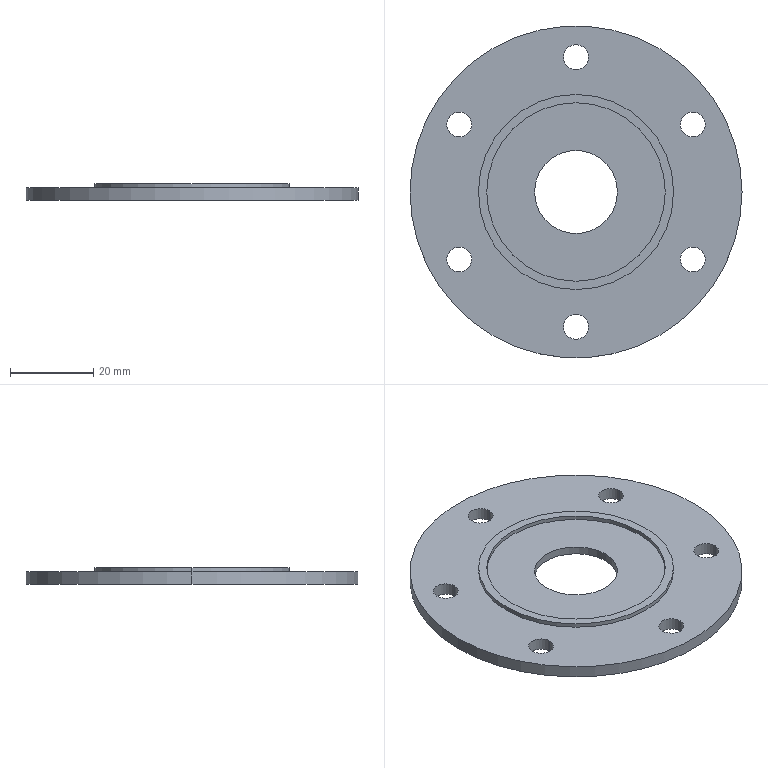Part | SolidWorks | features ICE 4, Chamfer 1, CirPattern 1, Extrusion 1 | 1 solid | 27 faces | box 80 x 80 x 4 mm | volume 12563 mm3 | cylinder 20 | plane 5 | cone 2 | commonest cylinder face diameters 6 x12 20 x2 43 x2 47 x2 80 x2
STEP:
#1=CARTESIAN_POINT('',(22.5,0.,1.));
#2=VERTEX_POINT('',#1);
#3=CARTESIAN_POINT('',(-22.5,0.,1.));
#4=VERTEX_POINT('',#3);
#5=CARTESIAN_POINT('',(0.,0.,1.));
#6=DIRECTION('',(0.,0.,-1.));
#7=DIRECTION('',(-1.,0.,0.));
#8=AXIS2_PLACEMENT_3D('',#5,#6,#7);
#9=CIRCLE('',#8,22.5);
#10=EDGE_CURVE('',#2,#4,#9,.T.);
#11=ORIENTED_EDGE('',*,*,#10,.F.);
#12=CARTESIAN_POINT('',(23.5,0.,0.));
#13=VERTEX_POINT('',#12);
#14=CARTESIAN_POINT('',(22.5,0.,1.));
#15=DIRECTION('',(0.7071,0.,-0.7071));
#16=VECTOR('',#15,1000.);
#17=LINE('',#14,#16);
#18=EDGE_CURVE('',#2,#13,#17,.T.);
#19=ORIENTED_EDGE('',*,*,#18,.T.);
#20=CARTESIAN_POINT('',(-23.5,0.,0.));
#21=VERTEX_POINT('',#20);
#22=CARTESIAN_POINT('',(0.,0.,0.));
#23=DIRECTION('',(0.,0.,-1.));
#24=DIRECTION('',(-1.,0.,0.));
#25=AXIS2_PLACEMENT_3D('',#22,#23,#24);
#26=CIRCLE('',#25,23.5);
#27=EDGE_CURVE('',#13,#21,#26,.T.);
#28=ORIENTED_EDGE('',*,*,#27,.T.);
#29=CARTESIAN_POINT('',(-22.5,0.,1.));
#30=DIRECTION('',(-0.7071,0.,-0.7071));
#31=VECTOR('',#30,1000.);
#32=LINE('',#29,#31);
#33=EDGE_CURVE('',#4,#21,#32,.T.);
#34=ORIENTED_EDGE('',*,*,#33,.F.);
#35=EDGE_LOOP('',(#11,#19,#28,#34));
#36=FACE_OUTER_BOUND('',#35,.T.);
#37=CARTESIAN_POINT('',(0.,0.,1.));
#38=DIRECTION('',(0.,0.,-1.));
#39=DIRECTION('',(-1.,0.,0.));
#40=AXIS2_PLACEMENT_3D('',#37,#38,#39);
#41=CONICAL_SURFACE('',#40,22.5,0.7854);
#42=ADVANCED_FACE('',(#36),#41,.F.);
#43=CARTESIAN_POINT('',(-31.146,16.25,3.));
#44=VERTEX_POINT('',#43);
#45=CARTESIAN_POINT('',(-25.146,16.25,3.));
#46=VERTEX_POINT('',#45);
#47=CARTESIAN_POINT('',(-28.146,16.25,3.));
#48=DIRECTION('',(0.,0.,1.));
#49=DIRECTION('',(1.,0.,0.));
#50=AXIS2_PLACEMENT_3D('',#47,#48,#49);
#51=CIRCLE('',#50,3.);
#52=EDGE_CURVE('',#44,#46,#51,.T.);
#53=ORIENTED_EDGE('',*,*,#52,.T.);
#54=CARTESIAN_POINT('',(-25.146,16.25,0.));
#55=VERTEX_POINT('',#54);
#56=CARTESIAN_POINT('',(-25.146,16.25,4.));
#57=DIRECTION('',(0.,0.,-1.));
#58=VECTOR('',#57,1000.);
#59=LINE('',#56,#58);
#60=EDGE_CURVE('',#46,#55,#59,.T.);
#61=ORIENTED_EDGE('',*,*,#60,.T.);
#62=CARTESIAN_POINT('',(-31.146,16.25,0.));
#63=VERTEX_POINT('',#62);
#64=CARTESIAN_POINT('',(-28.146,16.25,0.));
#65=DIRECTION('',(0.,0.,-1.));
#66=DIRECTION('',(-0.5,-0.866,0.));
#67=AXIS2_PLACEMENT_3D('',#64,#65,#66);
#68=CIRCLE('',#67,3.);
#69=EDGE_CURVE('',#55,#63,#68,.T.);
#70=ORIENTED_EDGE('',*,*,#69,.T.);
#71=CARTESIAN_POINT('',(-31.146,16.25,4.));
#72=DIRECTION('',(0.,0.,-1.));
#73=VECTOR('',#72,1000.);
#74=LINE('',#71,#73);
#75=EDGE_CURVE('',#44,#63,#74,.T.);
#76=ORIENTED_EDGE('',*,*,#75,.F.);
#77=EDGE_LOOP('',(#53,#61,#70,#76));
#78=FACE_OUTER_BOUND('',#77,.T.);
#79=CARTESIAN_POINT('',(-28.146,16.25,4.));
#80=DIRECTION('',(0.,0.,-1.));
#81=DIRECTION('',(-1.,0.,0.));
#82=AXIS2_PLACEMENT_3D('',#79,#80,#81);
#83=CYLINDRICAL_SURFACE('',#82,3.);
#84=ADVANCED_FACE('',(#78),#83,.F.);
#85=CARTESIAN_POINT('',(-31.146,-16.25,3.));
#86=VERTEX_POINT('',#85);
#87=CARTESIAN_POINT('',(-25.146,-16.25,3.));
#88=VERTEX_POINT('',#87);
#89=CARTESIAN_POINT('',(-28.146,-16.25,3.));
#90=DIRECTION('',(0.,0.,1.));
#91=DIRECTION('',(1.,0.,0.));
#92=AXIS2_PLACEMENT_3D('',#89,#90,#91);
#93=CIRCLE('',#92,3.);
#94=EDGE_CURVE('',#86,#88,#93,.T.);
#95=ORIENTED_EDGE('',*,*,#94,.T.);
#96=CARTESIAN_POINT('',(-25.146,-16.25,0.));
#97=VERTEX_POINT('',#96);
#98=CARTESIAN_POINT('',(-25.146,-16.25,4.));
#99=DIRECTION('',(0.,0.,-1.));
#100=VECTOR('',#99,1000.);
#101=LINE('',#98,#100);
#102=EDGE_CURVE('',#88,#97,#101,.T.);
#103=ORIENTED_EDGE('',*,*,#102,.T.);
#104=CARTESIAN_POINT('',(-31.146,-16.25,0.));
#105=VERTEX_POINT('',#104);
#106=CARTESIAN_POINT('',(-28.146,-16.25,0.));
#107=DIRECTION('',(0.,0.,-1.));
#108=DIRECTION('',(0.5,-0.866,0.));
#109=AXIS2_PLACEMENT_3D('',#106,#107,#108);
#110=CIRCLE('',#109,3.);
#111=EDGE_CURVE('',#97,#105,#110,.T.);
#112=ORIENTED_EDGE('',*,*,#111,.T.);
#113=CARTESIAN_POINT('',(-31.146,-16.25,4.));
#114=DIRECTION('',(0.,0.,-1.));
#115=VECTOR('',#114,1000.);
#116=LINE('',#113,#115);
#117=EDGE_CURVE('',#86,#105,#116,.T.);
#118=ORIENTED_EDGE('',*,*,#117,.F.);
#119=EDGE_LOOP('',(#95,#103,#112,#118));
#120=FACE_OUTER_BOUND('',#119,.T.);
#121=CARTESIAN_POINT('',(-28.146,-16.25,4.));
#122=DIRECTION('',(0.,0.,-1.));
#123=DIRECTION('',(-1.,0.,0.));
#124=AXIS2_PLACEMENT_3D('',#121,#122,#123);
#125=CYLINDRICAL_SURFACE('',#124,3.);
#126=ADVANCED_FACE('',(#120),#125,.F.);
#127=CARTESIAN_POINT('',(-3.,-32.5,3.));
#128=VERTEX_POINT('',#127);
#129=CARTESIAN_POINT('',(3.,-32.5,3.));
#130=VERTEX_POINT('',#129);
#131=CARTESIAN_POINT('',(0.,-32.5,3.));
#132=DIRECTION('',(0.,0.,1.));
#133=DIRECTION('',(1.,0.,0.));
#134=AXIS2_PLACEMENT_3D('',#131,#132,#133);
#135=CIRCLE('',#134,3.);
#136=EDGE_CURVE('',#128,#130,#135,.T.);
#137=ORIENTED_EDGE('',*,*,#136,.T.);
#138=CARTESIAN_POINT('',(3.,-32.5,0.));
#139=VERTEX_POINT('',#138);
#140=CARTESIAN_POINT('',(3.,-32.5,4.));
#141=DIRECTION('',(0.,0.,-1.));
#142=VECTOR('',#141,1000.);
#143=LINE('',#140,#142);
#144=EDGE_CURVE('',#130,#139,#143,.T.);
#145=ORIENTED_EDGE('',*,*,#144,.T.);
#146=CARTESIAN_POINT('',(-3.,-32.5,0.));
#147=VERTEX_POINT('',#146);
#148=CARTESIAN_POINT('',(0.,-32.5,0.));
#149=DIRECTION('',(0.,0.,-1.));
#150=DIRECTION('',(1.,0.,0.));
#151=AXIS2_PLACEMENT_3D('',#148,#149,#150);
#152=CIRCLE('',#151,3.);
#153=EDGE_CURVE('',#139,#147,#152,.T.);
#154=ORIENTED_EDGE('',*,*,#153,.T.);
#155=CARTESIAN_POINT('',(-3.,-32.5,4.));
#156=DIRECTION('',(0.,0.,-1.));
#157=VECTOR('',#156,1000.);
#158=LINE('',#155,#157);
#159=EDGE_CURVE('',#128,#147,#158,.T.);
#160=ORIENTED_EDGE('',*,*,#159,.F.);
#161=EDGE_LOOP('',(#137,#145,#154,#160));
#162=FACE_OUTER_BOUND('',#161,.T.);
#163=CARTESIAN_POINT('',(0.,-32.5,4.));
#164=DIRECTION('',(0.,0.,-1.));
#165=DIRECTION('',(-1.,0.,0.));
#166=AXIS2_PLACEMENT_3D('',#163,#164,#165);
#167=CYLINDRICAL_SURFACE('',#166,3.);
#168=ADVANCED_FACE('',(#162),#167,.F.);
#169=CARTESIAN_POINT('',(25.146,-16.25,3.));
#170=VERTEX_POINT('',#169);
#171=CARTESIAN_POINT('',(31.146,-16.25,3.));
#172=VERTEX_POINT('',#171);
#173=CARTESIAN_POINT('',(28.146,-16.25,3.));
#174=DIRECTION('',(0.,0.,1.));
#175=DIRECTION('',(1.,0.,0.));
#176=AXIS2_PLACEMENT_3D('',#173,#174,#175);
#177=CIRCLE('',#176,3.);
#178=EDGE_CURVE('',#170,#172,#177,.T.);
#179=ORIENTED_EDGE('',*,*,#178,.T.);
#180=CARTESIAN_POINT('',(31.146,-16.25,0.));
#181=VERTEX_POINT('',#180);
#182=CARTESIAN_POINT('',(31.146,-16.25,4.));
#183=DIRECTION('',(0.,0.,-1.));
#184=VECTOR('',#183,1000.);
#185=LINE('',#182,#184);
#186=EDGE_CURVE('',#172,#181,#185,.T.);
#187=ORIENTED_EDGE('',*,*,#186,.T.);
#188=CARTESIAN_POINT('',(25.146,-16.25,0.));
#189=VERTEX_POINT('',#188);
#190=CARTESIAN_POINT('',(28.146,-16.25,0.));
#191=DIRECTION('',(0.,0.,-1.));
#192=DIRECTION('',(0.5,0.866,0.));
#193=AXIS2_PLACEMENT_3D('',#190,#191,#192);
#194=CIRCLE('',#193,3.);
#195=EDGE_CURVE('',#181,#189,#194,.T.);
#196=ORIENTED_EDGE('',*,*,#195,.T.);
#197=CARTESIAN_POINT('',(25.146,-16.25,4.));
#198=DIRECTION('',(0.,0.,-1.));
#199=VECTOR('',#198,1000.);
#200=LINE('',#197,#199);
#201=EDGE_CURVE('',#170,#189,#200,.T.);
#202=ORIENTED_EDGE('',*,*,#201,.F.);
#203=EDGE_LOOP('',(#179,#187,#196,#202));
#204=FACE_OUTER_BOUND('',#203,.T.);
#205=CARTESIAN_POINT('',(28.146,-16.25,4.));
#206=DIRECTION('',(0.,0.,-1.));
#207=DIRECTION('',(-1.,0.,0.));
#208=AXIS2_PLACEMENT_3D('',#205,#206,#207);
#209=CYLINDRICAL_SURFACE('',#208,3.);
#210=ADVANCED_FACE('',(#204),#209,.F.);
#211=CARTESIAN_POINT('',(25.146,16.25,3.));
#212=VERTEX_POINT('',#211);
#213=CARTESIAN_POINT('',(31.146,16.25,3.));
#214=VERTEX_POINT('',#213);
#215=CARTESIAN_POINT('',(28.146,16.25,3.));
#216=DIRECTION('',(0.,0.,1.));
#217=DIRECTION('',(1.,0.,0.));
#218=AXIS2_PLACEMENT_3D('',#215,#216,#217);
#219=CIRCLE('',#218,3.);
#220=EDGE_CURVE('',#212,#214,#219,.T.);
#221=ORIENTED_EDGE('',*,*,#220,.T.);
#222=CARTESIAN_POINT('',(31.146,16.25,0.));
#223=VERTEX_POINT('',#222);
#224=CARTESIAN_POINT('',(31.146,16.25,4.));
#225=DIRECTION('',(0.,0.,-1.));
#226=VECTOR('',#225,1000.);
#227=LINE('',#224,#226);
#228=EDGE_CURVE('',#214,#223,#227,.T.);
#229=ORIENTED_EDGE('',*,*,#228,.T.);
#230=CARTESIAN_POINT('',(25.146,16.25,0.));
#231=VERTEX_POINT('',#230);
#232=CARTESIAN_POINT('',(28.146,16.25,0.));
#233=DIRECTION('',(0.,0.,-1.));
#234=DIRECTION('',(-0.5,0.866,0.));
#235=AXIS2_PLACEMENT_3D('',#232,#233,#234);
#236=CIRCLE('',#235,3.);
#237=EDGE_CURVE('',#223,#231,#236,.T.);
#238=ORIENTED_EDGE('',*,*,#237,.T.);
#239=CARTESIAN_POINT('',(25.146,16.25,4.));
#240=DIRECTION('',(0.,0.,-1.));
#241=VECTOR('',#240,1000.);
#242=LINE('',#239,#241);
#243=EDGE_CURVE('',#212,#231,#242,.T.);
#244=ORIENTED_EDGE('',*,*,#243,.F.);
#245=EDGE_LOOP('',(#221,#229,#238,#244));
#246=FACE_OUTER_BOUND('',#245,.T.);
#247=CARTESIAN_POINT('',(28.146,16.25,4.));
#248=DIRECTION('',(0.,0.,-1.));
#249=DIRECTION('',(-1.,0.,0.));
#250=AXIS2_PLACEMENT_3D('',#247,#248,#249);
#251=CYLINDRICAL_SURFACE('',#250,3.);
#252=ADVANCED_FACE('',(#246),#251,.F.);
#253=CARTESIAN_POINT('',(-3.,32.5,3.));
#254=VERTEX_POINT('',#253);
#255=CARTESIAN_POINT('',(3.,32.5,3.));
#256=VERTEX_POINT('',#255);
#257=CARTESIAN_POINT('',(0.,32.5,3.));
#258=DIRECTION('',(0.,0.,1.));
#259=DIRECTION('',(1.,0.,0.));
#260=AXIS2_PLACEMENT_3D('',#257,#258,#259);
#261=CIRCLE('',#260,3.);
#262=EDGE_CURVE('',#254,#256,#261,.T.);
#263=ORIENTED_EDGE('',*,*,#262,.T.);
#264=CARTESIAN_POINT('',(3.,32.5,0.));
#265=VERTEX_POINT('',#264);
#266=CARTESIAN_POINT('',(3.,32.5,4.));
#267=DIRECTION('',(0.,0.,-1.));
#268=VECTOR('',#267,1000.);
#269=LINE('',#266,#268);
#270=EDGE_CURVE('',#256,#265,#269,.T.);
#271=ORIENTED_EDGE('',*,*,#270,.T.);
#272=CARTESIAN_POINT('',(-3.,32.5,0.));
#273=VERTEX_POINT('',#272);
#274=CARTESIAN_POINT('',(0.,32.5,0.));
#275=DIRECTION('',(0.,0.,-1.));
#276=DIRECTION('',(-1.,0.,0.));
#277=AXIS2_PLACEMENT_3D('',#274,#275,#276);
#278=CIRCLE('',#277,3.);
#279=EDGE_CURVE('',#265,#273,#278,.T.);
#280=ORIENTED_EDGE('',*,*,#279,.T.);
#281=CARTESIAN_POINT('',(-3.,32.5,4.));
#282=DIRECTION('',(0.,0.,-1.));
#283=VECTOR('',#282,1000.);
#284=LINE('',#281,#283);
#285=EDGE_CURVE('',#254,#273,#284,.T.);
#286=ORIENTED_EDGE('',*,*,#285,.F.);
#287=EDGE_LOOP('',(#263,#271,#280,#286));
#288=FACE_OUTER_BOUND('',#287,.T.);
#289=CARTESIAN_POINT('',(0.,32.5,4.));
#290=DIRECTION('',(0.,0.,-1.));
#291=DIRECTION('',(-1.,0.,0.));
#292=AXIS2_PLACEMENT_3D('',#289,#290,#291);
#293=CYLINDRICAL_SURFACE('',#292,3.);
#294=ADVANCED_FACE('',(#288),#293,.F.);
#295=CARTESIAN_POINT('',(-21.5,0.,4.));
#296=VERTEX_POINT('',#295);
#297=CARTESIAN_POINT('',(21.5,0.,4.));
#298=VERTEX_POINT('',#297);
#299=CARTESIAN_POINT('',(0.,0.,4.));
#300=DIRECTION('',(0.,0.,1.));
#301=DIRECTION('',(1.,0.,0.));
#302=AXIS2_PLACEMENT_3D('',#299,#300,#301);
#303=CIRCLE('',#302,21.5);
#304=EDGE_CURVE('',#296,#298,#303,.T.);
#305=ORIENTED_EDGE('',*,*,#304,.T.);
#306=CARTESIAN_POINT('',(21.5,0.,3.));
#307=VERTEX_POINT('',#306);
#308=CARTESIAN_POINT('',(21.5,0.,4.));
#309=DIRECTION('',(0.,0.,-1.));
#310=VECTOR('',#309,1000.);
#311=LINE('',#308,#310);
#312=EDGE_CURVE('',#298,#307,#311,.T.);
#313=ORIENTED_EDGE('',*,*,#312,.T.);
#314=CARTESIAN_POINT('',(-21.5,0.,3.));
#315=VERTEX_POINT('',#314);
#316=CARTESIAN_POINT('',(0.,0.,3.));
#317=DIRECTION('',(0.,0.,-1.));
#318=DIRECTION('',(1.,0.,0.));
#319=AXIS2_PLACEMENT_3D('',#316,#317,#318);
#320=CIRCLE('',#319,21.5);
#321=EDGE_CURVE('',#307,#315,#320,.T.);
#322=ORIENTED_EDGE('',*,*,#321,.T.);
#323=CARTESIAN_POINT('',(-21.5,0.,4.));
#324=DIRECTION('',(0.,0.,-1.));
#325=VECTOR('',#324,1000.);
#326=LINE('',#323,#325);
#327=EDGE_CURVE('',#296,#315,#326,.T.);
#328=ORIENTED_EDGE('',*,*,#327,.F.);
#329=EDGE_LOOP('',(#305,#313,#322,#328));
#330=FACE_OUTER_BOUND('',#329,.T.);
#331=CARTESIAN_POINT('',(0.,0.,4.));
#332=DIRECTION('',(0.,0.,-1.));
#333=DIRECTION('',(-1.,0.,0.));
#334=AXIS2_PLACEMENT_3D('',#331,#332,#333);
#335=CYLINDRICAL_SURFACE('',#334,21.5);
#336=ADVANCED_FACE('',(#330),#335,.F.);
#337=CARTESIAN_POINT('',(23.5,0.,4.));
#338=VERTEX_POINT('',#337);
#339=CARTESIAN_POINT('',(-23.5,0.,4.));
#340=VERTEX_POINT('',#339);
#341=CARTESIAN_POINT('',(0.,0.,4.));
#342=DIRECTION('',(0.,0.,1.));
#343=DIRECTION('',(1.,0.,0.));
#344=AXIS2_PLACEMENT_3D('',#341,#342,#343);
#345=CIRCLE('',#344,23.5);
#346=EDGE_CURVE('',#338,#340,#345,.T.);
#347=ORIENTED_EDGE('',*,*,#346,.F.);
#348=CARTESIAN_POINT('',(23.5,0.,3.));
#349=VERTEX_POINT('',#348);
#350=CARTESIAN_POINT('',(23.5,0.,4.));
#351=DIRECTION('',(0.,0.,-1.));
#352=VECTOR('',#351,1000.);
#353=LINE('',#350,#352);
#354=EDGE_CURVE('',#338,#349,#353,.T.);
#355=ORIENTED_EDGE('',*,*,#354,.T.);
#356=CARTESIAN_POINT('',(-23.5,0.,3.));
#357=VERTEX_POINT('',#356);
#358=CARTESIAN_POINT('',(0.,0.,3.));
#359=DIRECTION('',(0.,0.,1.));
#360=DIRECTION('',(1.,0.,0.));
#361=AXIS2_PLACEMENT_3D('',#358,#359,#360);
#362=CIRCLE('',#361,23.5);
#363=EDGE_CURVE('',#349,#357,#362,.T.);
#364=ORIENTED_EDGE('',*,*,#363,.T.);
#365=CARTESIAN_POINT('',(-23.5,0.,4.));
#366=DIRECTION('',(0.,0.,-1.));
#367=VECTOR('',#366,1000.);
#368=LINE('',#365,#367);
#369=EDGE_CURVE('',#340,#357,#368,.T.);
#370=ORIENTED_EDGE('',*,*,#369,.F.);
#371=EDGE_LOOP('',(#347,#355,#364,#370));
#372=FACE_OUTER_BOUND('',#371,.T.);
#373=CARTESIAN_POINT('',(0.,0.,4.));
#374=DIRECTION('',(0.,0.,-1.));
#375=DIRECTION('',(-1.,0.,0.));
#376=AXIS2_PLACEMENT_3D('',#373,#374,#375);
#377=CYLINDRICAL_SURFACE('',#376,23.5);
#378=ADVANCED_FACE('',(#372),#377,.T.);
#379=CARTESIAN_POINT('',(40.,0.,3.));
#380=VERTEX_POINT('',#379);
#381=CARTESIAN_POINT('',(-40.,0.,3.));
#382=VERTEX_POINT('',#381);
#383=CARTESIAN_POINT('',(0.,0.,3.));
#384=DIRECTION('',(0.,0.,1.));
#385=DIRECTION('',(1.,0.,0.));
#386=AXIS2_PLACEMENT_3D('',#383,#384,#385);
#387=CIRCLE('',#386,40.);
#388=EDGE_CURVE('',#380,#382,#387,.T.);
#389=ORIENTED_EDGE('',*,*,#388,.F.);
#390=CARTESIAN_POINT('',(40.,0.,0.));
#391=VERTEX_POINT('',#390);
#392=CARTESIAN_POINT('',(40.,0.,3.));
#393=DIRECTION('',(0.,0.,-1.));
#394=VECTOR('',#393,1000.);
#395=LINE('',#392,#394);
#396=EDGE_CURVE('',#380,#391,#395,.T.);
#397=ORIENTED_EDGE('',*,*,#396,.T.);
#398=CARTESIAN_POINT('',(-40.,0.,0.));
#399=VERTEX_POINT('',#398);
#400=CARTESIAN_POINT('',(0.,0.,0.));
#401=DIRECTION('',(0.,0.,1.));
#402=DIRECTION('',(1.,0.,0.));
#403=AXIS2_PLACEMENT_3D('',#400,#401,#402);
#404=CIRCLE('',#403,40.);
#405=EDGE_CURVE('',#391,#399,#404,.T.);
#406=ORIENTED_EDGE('',*,*,#405,.T.);
#407=CARTESIAN_POINT('',(-40.,0.,3.));
#408=DIRECTION('',(0.,0.,-1.));
#409=VECTOR('',#408,1000.);
#410=LINE('',#407,#409);
#411=EDGE_CURVE('',#382,#399,#410,.T.);
#412=ORIENTED_EDGE('',*,*,#411,.F.);
#413=EDGE_LOOP('',(#389,#397,#406,#412));
#414=FACE_OUTER_BOUND('',#413,.T.);
#415=CARTESIAN_POINT('',(0.,0.,3.));
#416=DIRECTION('',(0.,0.,-1.));
#417=DIRECTION('',(-1.,0.,0.));
#418=AXIS2_PLACEMENT_3D('',#415,#416,#417);
#419=CYLINDRICAL_SURFACE('',#418,40.);
#420=ADVANCED_FACE('',(#414),#419,.T.);
#421=CARTESIAN_POINT('',(-10.,0.,1.));
#422=VERTEX_POINT('',#421);
#423=CARTESIAN_POINT('',(10.,0.,1.));
#424=VERTEX_POINT('',#423);
#425=CARTESIAN_POINT('',(0.,0.,1.));
#426=DIRECTION('',(0.,0.,1.));
#427=DIRECTION('',(-1.,0.,0.));
#428=AXIS2_PLACEMENT_3D('',#425,#426,#427);
#429=CIRCLE('',#428,10.);
#430=EDGE_CURVE('',#422,#424,#429,.T.);
#431=ORIENTED_EDGE('',*,*,#430,.F.);
#432=CARTESIAN_POINT('',(-10.,0.,3.));
#433=VERTEX_POINT('',#432);
#434=CARTESIAN_POINT('',(-10.,0.,0.));
#435=DIRECTION('',(0.,0.,1.));
#436=VECTOR('',#435,1000.);
#437=LINE('',#434,#436);
#438=EDGE_CURVE('',#422,#433,#437,.T.);
#439=ORIENTED_EDGE('',*,*,#438,.T.);
#440=CARTESIAN_POINT('',(10.,0.,3.));
#441=VERTEX_POINT('',#440);
#442=CARTESIAN_POINT('',(0.,0.,3.));
#443=DIRECTION('',(0.,0.,1.));
#444=DIRECTION('',(1.,0.,0.));
#445=AXIS2_PLACEMENT_3D('',#442,#443,#444);
#446=CIRCLE('',#445,10.);
#447=EDGE_CURVE('',#433,#441,#446,.T.);
#448=ORIENTED_EDGE('',*,*,#447,.T.);
#449=CARTESIAN_POINT('',(10.,0.,0.));
#450=DIRECTION('',(0.,0.,1.));
#451=VECTOR('',#450,1000.);
#452=LINE('',#449,#451);
#453=EDGE_CURVE('',#424,#441,#452,.T.);
#454=ORIENTED_EDGE('',*,*,#453,.F.);
#455=EDGE_LOOP('',(#431,#439,#448,#454));
#456=FACE_OUTER_BOUND('',#455,.T.);
#457=CARTESIAN_POINT('',(0.,0.,0.));
#458=DIRECTION('',(0.,0.,1.));
#459=DIRECTION('',(1.,0.,0.));
#460=AXIS2_PLACEMENT_3D('',#457,#458,#459);
#461=CYLINDRICAL_SURFACE('',#460,10.);
#462=ADVANCED_FACE('',(#456),#461,.F.);
#463=ORIENTED_EDGE('',*,*,#438,.F.);
#464=CARTESIAN_POINT('',(0.,0.,1.));
#465=DIRECTION('',(0.,0.,1.));
#466=DIRECTION('',(-1.,0.,0.));
#467=AXIS2_PLACEMENT_3D('',#464,#465,#466);
#468=CIRCLE('',#467,10.);
#469=EDGE_CURVE('',#424,#422,#468,.T.);
#470=ORIENTED_EDGE('',*,*,#469,.F.);
#471=ORIENTED_EDGE('',*,*,#453,.T.);
#472=CARTESIAN_POINT('',(0.,0.,3.));
#473=DIRECTION('',(0.,0.,1.));
#474=DIRECTION('',(1.,0.,0.));
#475=AXIS2_PLACEMENT_3D('',#472,#473,#474);
#476=CIRCLE('',#475,10.);
#477=EDGE_CURVE('',#441,#433,#476,.T.);
#478=ORIENTED_EDGE('',*,*,#477,.T.);
#479=EDGE_LOOP('',(#463,#470,#471,#478));
#480=FACE_OUTER_BOUND('',#479,.T.);
#481=CARTESIAN_POINT('',(0.,0.,0.));
#482=DIRECTION('',(0.,0.,1.));
#483=DIRECTION('',(1.,0.,0.));
#484=AXIS2_PLACEMENT_3D('',#481,#482,#483);
#485=CYLINDRICAL_SURFACE('',#484,10.);
#486=ADVANCED_FACE('',(#480),#485,.F.);
#487=ORIENTED_EDGE('',*,*,#52,.F.);
#488=CARTESIAN_POINT('',(-28.146,16.25,3.));
#489=DIRECTION('',(0.,0.,1.));
#490=DIRECTION('',(1.,0.,0.));
#491=AXIS2_PLACEMENT_3D('',#488,#489,#490);
#492=CIRCLE('',#491,3.);
#493=EDGE_CURVE('',#46,#44,#492,.T.);
#494=ORIENTED_EDGE('',*,*,#493,.F.);
#495=EDGE_LOOP('',(#487,#494));
#496=FACE_BOUND('',#495,.T.);
#497=ORIENTED_EDGE('',*,*,#94,.F.);
#498=CARTESIAN_POINT('',(-28.146,-16.25,3.));
#499=DIRECTION('',(0.,0.,1.));
#500=DIRECTION('',(1.,0.,0.));
#501=AXIS2_PLACEMENT_3D('',#498,#499,#500);
#502=CIRCLE('',#501,3.);
#503=EDGE_CURVE('',#88,#86,#502,.T.);
#504=ORIENTED_EDGE('',*,*,#503,.F.);
#505=EDGE_LOOP('',(#497,#504));
#506=FACE_BOUND('',#505,.T.);
#507=ORIENTED_EDGE('',*,*,#136,.F.);
#508=CARTESIAN_POINT('',(0.,-32.5,3.));
#509=DIRECTION('',(0.,0.,1.));
#510=DIRECTION('',(1.,0.,0.));
#511=AXIS2_PLACEMENT_3D('',#508,#509,#510);
#512=CIRCLE('',#511,3.);
#513=EDGE_CURVE('',#130,#128,#512,.T.);
#514=ORIENTED_EDGE('',*,*,#513,.F.);
#515=EDGE_LOOP('',(#507,#514));
#516=FACE_BOUND('',#515,.T.);
#517=ORIENTED_EDGE('',*,*,#178,.F.);
#518=CARTESIAN_POINT('',(28.146,-16.25,3.));
#519=DIRECTION('',(0.,0.,1.));
#520=DIRECTION('',(1.,0.,0.));
#521=AXIS2_PLACEMENT_3D('',#518,#519,#520);
#522=CIRCLE('',#521,3.);
#523=EDGE_CURVE('',#172,#170,#522,.T.);
#524=ORIENTED_EDGE('',*,*,#523,.F.);
#525=EDGE_LOOP('',(#517,#524));
#526=FACE_BOUND('',#525,.T.);
#527=ORIENTED_EDGE('',*,*,#220,.F.);
#528=CARTESIAN_POINT('',(28.146,16.25,3.));
#529=DIRECTION('',(0.,0.,1.));
#530=DIRECTION('',(1.,0.,0.));
#531=AXIS2_PLACEMENT_3D('',#528,#529,#530);
#532=CIRCLE('',#531,3.);
#533=EDGE_CURVE('',#214,#212,#532,.T.);
#534=ORIENTED_EDGE('',*,*,#533,.F.);
#535=EDGE_LOOP('',(#527,#534));
#536=FACE_BOUND('',#535,.T.);
#537=ORIENTED_EDGE('',*,*,#262,.F.);
#538=CARTESIAN_POINT('',(0.,32.5,3.));
#539=DIRECTION('',(0.,0.,1.));
#540=DIRECTION('',(1.,0.,0.));
#541=AXIS2_PLACEMENT_3D('',#538,#539,#540);
#542=CIRCLE('',#541,3.);
#543=EDGE_CURVE('',#256,#254,#542,.T.);
#544=ORIENTED_EDGE('',*,*,#543,.F.);
#545=EDGE_LOOP('',(#537,#544));
#546=FACE_BOUND('',#545,.T.);
#547=CARTESIAN_POINT('',(0.,0.,3.));
#548=DIRECTION('',(0.,0.,1.));
#549=DIRECTION('',(1.,0.,0.));
#550=AXIS2_PLACEMENT_3D('',#547,#548,#549);
#551=CIRCLE('',#550,40.);
#552=EDGE_CURVE('',#382,#380,#551,.T.);
#553=ORIENTED_EDGE('',*,*,#552,.T.);
#554=ORIENTED_EDGE('',*,*,#388,.T.);
#555=EDGE_LOOP('',(#553,#554));
#556=FACE_OUTER_BOUND('',#555,.T.);
#557=CARTESIAN_POINT('',(0.,0.,3.));
#558=DIRECTION('',(0.,0.,1.));
#559=DIRECTION('',(1.,0.,0.));
#560=AXIS2_PLACEMENT_3D('',#557,#558,#559);
#561=CIRCLE('',#560,23.5);
#562=EDGE_CURVE('',#357,#349,#561,.T.);
#563=ORIENTED_EDGE('',*,*,#562,.F.);
#564=ORIENTED_EDGE('',*,*,#363,.F.);
#565=EDGE_LOOP('',(#563,#564));
#566=FACE_BOUND('',#565,.T.);
#567=CARTESIAN_POINT('',(0.,0.,3.));
#568=DIRECTION('',(0.,0.,1.));
#569=DIRECTION('',(1.,0.,0.));
#570=AXIS2_PLACEMENT_3D('',#567,#568,#569);
#571=PLANE('',#570);
#572=ADVANCED_FACE('',(#496,#506,#516,#526,#536,#546,#556,#566),#571,.T.);
#573=ORIENTED_EDGE('',*,*,#396,.F.);
#574=ORIENTED_EDGE('',*,*,#552,.F.);
#575=ORIENTED_EDGE('',*,*,#411,.T.);
#576=CARTESIAN_POINT('',(0.,0.,0.));
#577=DIRECTION('',(0.,0.,1.));
#578=DIRECTION('',(1.,0.,0.));
#579=AXIS2_PLACEMENT_3D('',#576,#577,#578);
#580=CIRCLE('',#579,40.);
#581=EDGE_CURVE('',#399,#391,#580,.T.);
#582=ORIENTED_EDGE('',*,*,#581,.T.);
#583=EDGE_LOOP('',(#573,#574,#575,#582));
#584=FACE_OUTER_BOUND('',#583,.T.);
#585=CARTESIAN_POINT('',(0.,0.,3.));
#586=DIRECTION('',(0.,0.,-1.));
#587=DIRECTION('',(-1.,0.,0.));
#588=AXIS2_PLACEMENT_3D('',#585,#586,#587);
#589=CYLINDRICAL_SURFACE('',#588,40.);
#590=ADVANCED_FACE('',(#584),#589,.T.);
#591=CARTESIAN_POINT('',(0.,0.,0.));
#592=DIRECTION('',(0.,0.,-1.));
#593=DIRECTION('',(-1.,0.,0.));
#594=AXIS2_PLACEMENT_3D('',#591,#592,#593);
#595=CIRCLE('',#594,23.5);
#596=EDGE_CURVE('',#21,#13,#595,.T.);
#597=ORIENTED_EDGE('',*,*,#596,.F.);
#598=ORIENTED_EDGE('',*,*,#27,.F.);
#599=EDGE_LOOP('',(#597,#598));
#600=FACE_BOUND('',#599,.T.);
#601=CARTESIAN_POINT('',(-28.146,16.25,0.));
#602=DIRECTION('',(0.,0.,-1.));
#603=DIRECTION('',(-0.5,-0.866,0.));
#604=AXIS2_PLACEMENT_3D('',#601,#602,#603);
#605=CIRCLE('',#604,3.);
#606=EDGE_CURVE('',#63,#55,#605,.T.);
#607=ORIENTED_EDGE('',*,*,#606,.F.);
#608=ORIENTED_EDGE('',*,*,#69,.F.);
#609=EDGE_LOOP('',(#607,#608));
#610=FACE_BOUND('',#609,.T.);
#611=CARTESIAN_POINT('',(-28.146,-16.25,0.));
#612=DIRECTION('',(0.,0.,-1.));
#613=DIRECTION('',(0.5,-0.866,0.));
#614=AXIS2_PLACEMENT_3D('',#611,#612,#613);
#615=CIRCLE('',#614,3.);
#616=EDGE_CURVE('',#105,#97,#615,.T.);
#617=ORIENTED_EDGE('',*,*,#616,.F.);
#618=ORIENTED_EDGE('',*,*,#111,.F.);
#619=EDGE_LOOP('',(#617,#618));
#620=FACE_BOUND('',#619,.T.);
#621=CARTESIAN_POINT('',(0.,-32.5,0.));
#622=DIRECTION('',(0.,0.,-1.));
#623=DIRECTION('',(1.,0.,0.));
#624=AXIS2_PLACEMENT_3D('',#621,#622,#623);
#625=CIRCLE('',#624,3.);
#626=EDGE_CURVE('',#147,#139,#625,.T.);
#627=ORIENTED_EDGE('',*,*,#626,.F.);
#628=ORIENTED_EDGE('',*,*,#153,.F.);
#629=EDGE_LOOP('',(#627,#628));
#630=FACE_BOUND('',#629,.T.);
#631=CARTESIAN_POINT('',(28.146,-16.25,0.));
#632=DIRECTION('',(0.,0.,-1.));
#633=DIRECTION('',(0.5,0.866,0.));
#634=AXIS2_PLACEMENT_3D('',#631,#632,#633);
#635=CIRCLE('',#634,3.);
#636=EDGE_CURVE('',#189,#181,#635,.T.);
#637=ORIENTED_EDGE('',*,*,#636,.F.);
#638=ORIENTED_EDGE('',*,*,#195,.F.);
#639=EDGE_LOOP('',(#637,#638));
#640=FACE_BOUND('',#639,.T.);
#641=CARTESIAN_POINT('',(28.146,16.25,0.));
#642=DIRECTION('',(0.,0.,-1.));
#643=DIRECTION('',(-0.5,0.866,0.));
#644=AXIS2_PLACEMENT_3D('',#641,#642,#643);
#645=CIRCLE('',#644,3.);
#646=EDGE_CURVE('',#231,#223,#645,.T.);
#647=ORIENTED_EDGE('',*,*,#646,.F.);
#648=ORIENTED_EDGE('',*,*,#237,.F.);
#649=EDGE_LOOP('',(#647,#648));
#650=FACE_BOUND('',#649,.T.);
#651=CARTESIAN_POINT('',(0.,32.5,0.));
#652=DIRECTION('',(0.,0.,-1.));
#653=DIRECTION('',(-1.,0.,0.));
#654=AXIS2_PLACEMENT_3D('',#651,#652,#653);
#655=CIRCLE('',#654,3.);
#656=EDGE_CURVE('',#273,#265,#655,.T.);
#657=ORIENTED_EDGE('',*,*,#656,.F.);
#658=ORIENTED_EDGE('',*,*,#279,.F.);
#659=EDGE_LOOP('',(#657,#658));
#660=FACE_BOUND('',#659,.T.);
#661=ORIENTED_EDGE('',*,*,#581,.F.);
#662=ORIENTED_EDGE('',*,*,#405,.F.);
#663=EDGE_LOOP('',(#661,#662));
#664=FACE_OUTER_BOUND('',#663,.T.);
#665=CARTESIAN_POINT('',(0.,0.,0.));
#666=DIRECTION('',(0.,0.,1.));
#667=DIRECTION('',(1.,0.,0.));
#668=AXIS2_PLACEMENT_3D('',#665,#666,#667);
#669=PLANE('',#668);
#670=ADVANCED_FACE('',(#600,#610,#620,#630,#640,#650,#660,#664),#669,.F.);
#671=CARTESIAN_POINT('',(0.,0.,4.));
#672=DIRECTION('',(0.,0.,1.));
#673=DIRECTION('',(1.,0.,0.));
#674=AXIS2_PLACEMENT_3D('',#671,#672,#673);
#675=CIRCLE('',#674,23.5);
#676=EDGE_CURVE('',#340,#338,#675,.T.);
#677=ORIENTED_EDGE('',*,*,#676,.T.);
#678=ORIENTED_EDGE('',*,*,#346,.T.);
#679=EDGE_LOOP('',(#677,#678));
#680=FACE_OUTER_BOUND('',#679,.T.);
#681=ORIENTED_EDGE('',*,*,#304,.F.);
#682=CARTESIAN_POINT('',(0.,0.,4.));
#683=DIRECTION('',(0.,0.,1.));
#684=DIRECTION('',(1.,0.,0.));
#685=AXIS2_PLACEMENT_3D('',#682,#683,#684);
#686=CIRCLE('',#685,21.5);
#687=EDGE_CURVE('',#298,#296,#686,.T.);
#688=ORIENTED_EDGE('',*,*,#687,.F.);
#689=EDGE_LOOP('',(#681,#688));
#690=FACE_BOUND('',#689,.T.);
#691=CARTESIAN_POINT('',(0.,0.,4.));
#692=DIRECTION('',(0.,0.,1.));
#693=DIRECTION('',(1.,0.,0.));
#694=AXIS2_PLACEMENT_3D('',#691,#692,#693);
#695=PLANE('',#694);
#696=ADVANCED_FACE('',(#680,#690),#695,.T.);
#697=ORIENTED_EDGE('',*,*,#354,.F.);
#698=ORIENTED_EDGE('',*,*,#676,.F.);
#699=ORIENTED_EDGE('',*,*,#369,.T.);
#700=ORIENTED_EDGE('',*,*,#562,.T.);
#701=EDGE_LOOP('',(#697,#698,#699,#700));
#702=FACE_OUTER_BOUND('',#701,.T.);
#703=CARTESIAN_POINT('',(0.,0.,4.));
#704=DIRECTION('',(0.,0.,-1.));
#705=DIRECTION('',(-1.,0.,0.));
#706=AXIS2_PLACEMENT_3D('',#703,#704,#705);
#707=CYLINDRICAL_SURFACE('',#706,23.5);
#708=ADVANCED_FACE('',(#702),#707,.T.);
#709=ORIENTED_EDGE('',*,*,#312,.F.);
#710=ORIENTED_EDGE('',*,*,#687,.T.);
#711=ORIENTED_EDGE('',*,*,#327,.T.);
#712=CARTESIAN_POINT('',(0.,0.,3.));
#713=DIRECTION('',(0.,0.,-1.));
#714=DIRECTION('',(1.,0.,0.));
#715=AXIS2_PLACEMENT_3D('',#712,#713,#714);
#716=CIRCLE('',#715,21.5);
#717=EDGE_CURVE('',#315,#307,#716,.T.);
#718=ORIENTED_EDGE('',*,*,#717,.T.);
#719=EDGE_LOOP('',(#709,#710,#711,#718));
#720=FACE_OUTER_BOUND('',#719,.T.);
#721=CARTESIAN_POINT('',(0.,0.,4.));
#722=DIRECTION('',(0.,0.,-1.));
#723=DIRECTION('',(-1.,0.,0.));
#724=AXIS2_PLACEMENT_3D('',#721,#722,#723);
#725=CYLINDRICAL_SURFACE('',#724,21.5);
#726=ADVANCED_FACE('',(#720),#725,.F.);
#727=ORIENTED_EDGE('',*,*,#477,.F.);
#728=ORIENTED_EDGE('',*,*,#447,.F.);
#729=EDGE_LOOP('',(#727,#728));
#730=FACE_BOUND('',#729,.T.);
#731=ORIENTED_EDGE('',*,*,#717,.F.);
#732=ORIENTED_EDGE('',*,*,#321,.F.);
#733=EDGE_LOOP('',(#731,#732));
#734=FACE_OUTER_BOUND('',#733,.T.);
#735=CARTESIAN_POINT('',(0.,0.,3.));
#736=DIRECTION('',(0.,0.,1.));
#737=DIRECTION('',(1.,0.,0.));
#738=AXIS2_PLACEMENT_3D('',#735,#736,#737);
#739=PLANE('',#738);
#740=ADVANCED_FACE('',(#730,#734),#739,.T.);
#741=ORIENTED_EDGE('',*,*,#270,.F.);
#742=ORIENTED_EDGE('',*,*,#543,.T.);
#743=ORIENTED_EDGE('',*,*,#285,.T.);
#744=ORIENTED_EDGE('',*,*,#656,.T.);
#745=EDGE_LOOP('',(#741,#742,#743,#744));
#746=FACE_OUTER_BOUND('',#745,.T.);
#747=CARTESIAN_POINT('',(0.,32.5,4.));
#748=DIRECTION('',(0.,0.,-1.));
#749=DIRECTION('',(-1.,0.,0.));
#750=AXIS2_PLACEMENT_3D('',#747,#748,#749);
#751=CYLINDRICAL_SURFACE('',#750,3.);
#752=ADVANCED_FACE('',(#746),#751,.F.);
#753=ORIENTED_EDGE('',*,*,#228,.F.);
#754=ORIENTED_EDGE('',*,*,#533,.T.);
#755=ORIENTED_EDGE('',*,*,#243,.T.);
#756=ORIENTED_EDGE('',*,*,#646,.T.);
#757=EDGE_LOOP('',(#753,#754,#755,#756));
#758=FACE_OUTER_BOUND('',#757,.T.);
#759=CARTESIAN_POINT('',(28.146,16.25,4.));
#760=DIRECTION('',(0.,0.,-1.));
#761=DIRECTION('',(-1.,0.,0.));
#762=AXIS2_PLACEMENT_3D('',#759,#760,#761);
#763=CYLINDRICAL_SURFACE('',#762,3.);
#764=ADVANCED_FACE('',(#758),#763,.F.);
#765=ORIENTED_EDGE('',*,*,#186,.F.);
#766=ORIENTED_EDGE('',*,*,#523,.T.);
#767=ORIENTED_EDGE('',*,*,#201,.T.);
#768=ORIENTED_EDGE('',*,*,#636,.T.);
#769=EDGE_LOOP('',(#765,#766,#767,#768));
#770=FACE_OUTER_BOUND('',#769,.T.);
#771=CARTESIAN_POINT('',(28.146,-16.25,4.));
#772=DIRECTION('',(0.,0.,-1.));
#773=DIRECTION('',(-1.,0.,0.));
#774=AXIS2_PLACEMENT_3D('',#771,#772,#773);
#775=CYLINDRICAL_SURFACE('',#774,3.);
#776=ADVANCED_FACE('',(#770),#775,.F.);
#777=ORIENTED_EDGE('',*,*,#144,.F.);
#778=ORIENTED_EDGE('',*,*,#513,.T.);
#779=ORIENTED_EDGE('',*,*,#159,.T.);
#780=ORIENTED_EDGE('',*,*,#626,.T.);
#781=EDGE_LOOP('',(#777,#778,#779,#780));
#782=FACE_OUTER_BOUND('',#781,.T.);
#783=CARTESIAN_POINT('',(0.,-32.5,4.));
#784=DIRECTION('',(0.,0.,-1.));
#785=DIRECTION('',(-1.,0.,0.));
#786=AXIS2_PLACEMENT_3D('',#783,#784,#785);
#787=CYLINDRICAL_SURFACE('',#786,3.);
#788=ADVANCED_FACE('',(#782),#787,.F.);
#789=ORIENTED_EDGE('',*,*,#102,.F.);
#790=ORIENTED_EDGE('',*,*,#503,.T.);
#791=ORIENTED_EDGE('',*,*,#117,.T.);
#792=ORIENTED_EDGE('',*,*,#616,.T.);
#793=EDGE_LOOP('',(#789,#790,#791,#792));
#794=FACE_OUTER_BOUND('',#793,.T.);
#795=CARTESIAN_POINT('',(-28.146,-16.25,4.));
#796=DIRECTION('',(0.,0.,-1.));
#797=DIRECTION('',(-1.,0.,0.));
#798=AXIS2_PLACEMENT_3D('',#795,#796,#797);
#799=CYLINDRICAL_SURFACE('',#798,3.);
#800=ADVANCED_FACE('',(#794),#799,.F.);
#801=ORIENTED_EDGE('',*,*,#60,.F.);
#802=ORIENTED_EDGE('',*,*,#493,.T.);
#803=ORIENTED_EDGE('',*,*,#75,.T.);
#804=ORIENTED_EDGE('',*,*,#606,.T.);
#805=EDGE_LOOP('',(#801,#802,#803,#804));
#806=FACE_OUTER_BOUND('',#805,.T.);
#807=CARTESIAN_POINT('',(-28.146,16.25,4.));
#808=DIRECTION('',(0.,0.,-1.));
#809=DIRECTION('',(-1.,0.,0.));
#810=AXIS2_PLACEMENT_3D('',#807,#808,#809);
#811=CYLINDRICAL_SURFACE('',#810,3.);
#812=ADVANCED_FACE('',(#806),#811,.F.);
#813=CARTESIAN_POINT('',(0.,0.,1.));
#814=DIRECTION('',(0.,0.,-1.));
#815=DIRECTION('',(-1.,0.,0.));
#816=AXIS2_PLACEMENT_3D('',#813,#814,#815);
#817=CIRCLE('',#816,22.5);
#818=EDGE_CURVE('',#4,#2,#817,.T.);
#819=ORIENTED_EDGE('',*,*,#818,.T.);
#820=ORIENTED_EDGE('',*,*,#10,.T.);
#821=EDGE_LOOP('',(#819,#820));
#822=FACE_OUTER_BOUND('',#821,.T.);
#823=ORIENTED_EDGE('',*,*,#469,.T.);
#824=ORIENTED_EDGE('',*,*,#430,.T.);
#825=EDGE_LOOP('',(#823,#824));
#826=FACE_BOUND('',#825,.T.);
#827=CARTESIAN_POINT('',(0.,0.,1.));
#828=DIRECTION('',(0.,0.,-1.));
#829=DIRECTION('',(-1.,0.,0.));
#830=AXIS2_PLACEMENT_3D('',#827,#828,#829);
#831=PLANE('',#830);
#832=ADVANCED_FACE('',(#822,#826),#831,.T.);
#833=ORIENTED_EDGE('',*,*,#18,.F.);
#834=ORIENTED_EDGE('',*,*,#818,.F.);
#835=ORIENTED_EDGE('',*,*,#33,.T.);
#836=ORIENTED_EDGE('',*,*,#596,.T.);
#837=EDGE_LOOP('',(#833,#834,#835,#836));
#838=FACE_OUTER_BOUND('',#837,.T.);
#839=CARTESIAN_POINT('',(0.,0.,1.));
#840=DIRECTION('',(0.,0.,-1.));
#841=DIRECTION('',(-1.,0.,0.));
#842=AXIS2_PLACEMENT_3D('',#839,#840,#841);
#843=CONICAL_SURFACE('',#842,22.5,0.7854);
#844=ADVANCED_FACE('',(#838),#843,.F.);
#845=CLOSED_SHELL('',(#42,#84,#126,#168,#210,#252,#294,#336,#378,#420,#462,#486,#572,#590,#670,#696,#708,#726,#740,#752,#764,#776,#788,#800,#812,#832,#844));
#846=MANIFOLD_SOLID_BREP('',#845);
#847=CARTESIAN_POINT('',(0.,0.,0.));
#848=DIRECTION('',(0.,0.,1.));
#849=DIRECTION('',(1.,0.,0.));
#850=AXIS2_PLACEMENT_3D('',#847,#848,#849);
#851=(LENGTH_UNIT()NAMED_UNIT(*)SI_UNIT(.MILLI.,.METRE.));
#852=UNCERTAINTY_MEASURE_WITH_UNIT(LENGTH_MEASURE(0.00001),#851,'','');
#853=(NAMED_UNIT(*)PLANE_ANGLE_UNIT()SI_UNIT($,.RADIAN.));
#854=(NAMED_UNIT(*)SI_UNIT($,.STERADIAN.)SOLID_ANGLE_UNIT());
#855=(GEOMETRIC_REPRESENTATION_CONTEXT(3)GLOBAL_UNCERTAINTY_ASSIGNED_CONTEXT((#852))GLOBAL_UNIT_ASSIGNED_CONTEXT((#851,#853,#854))REPRESENTATION_CONTEXT('',''));
#856=ADVANCED_BREP_SHAPE_REPRESENTATION('',(#846,#850),#855);